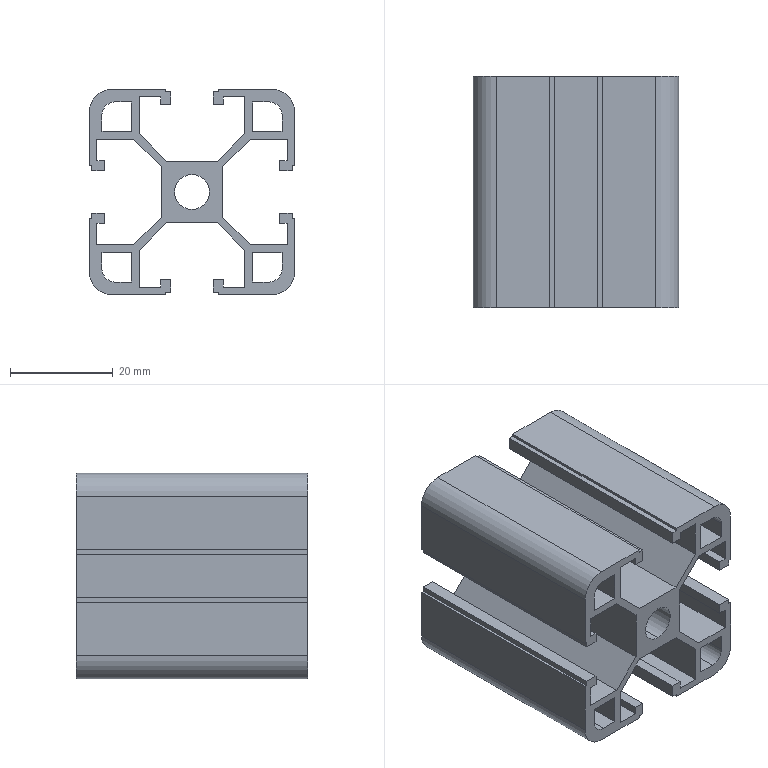Part | SolidWorks | features BaseBody 1 | 1 solid | 104 faces | box 40 x 45 x 40 mm | volume 21369 mm3 | plane 94 | cylinder 10 | commonest cylinder face diameters 5 x4 9 x4 6.8 x2